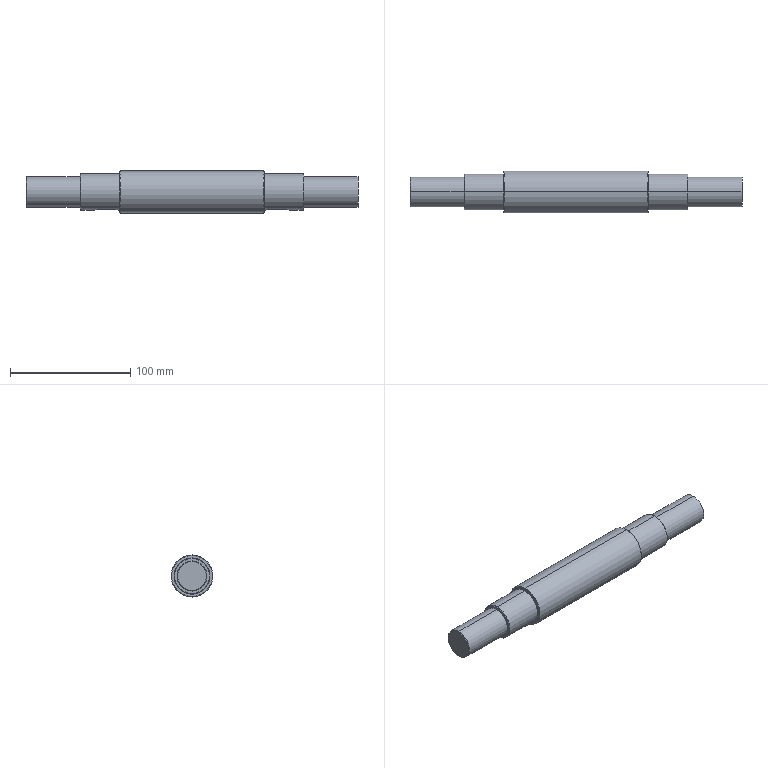Part | SolidWorks | features Chamfer 1, ICE 1, Revolution 1 | 1 solid | 38 faces | box 276 x 35 x 35 mm | volume 205103 mm3 | cylinder 16 | plane 12 | cone 10 | commonest cylinder face diameters 8 x6 25 x4 30 x4 35 x2
STEP:
#1=CARTESIAN_POINT('',(-65.,4.,-14.457));
#2=VERTEX_POINT('',#1);
#3=CARTESIAN_POINT('',(-61.,0.,-15.));
#4=VERTEX_POINT('',#3);
#5=CARTESIAN_POINT('',(-65.,4.,-14.457));
#6=CARTESIAN_POINT('',(-64.736,4.,-14.457));
#7=CARTESIAN_POINT('',(-64.476,3.974,-14.464));
#8=CARTESIAN_POINT('',(-63.962,3.872,-14.492));
#9=CARTESIAN_POINT('',(-63.707,3.794,-14.513));
#10=CARTESIAN_POINT('',(-63.224,3.594,-14.563));
#11=CARTESIAN_POINT('',(-62.995,3.471,-14.594));
#12=CARTESIAN_POINT('',(-62.558,3.179,-14.66));
#13=CARTESIAN_POINT('',(-62.356,3.013,-14.695));
#14=CARTESIAN_POINT('',(-61.989,2.646,-14.766));
#15=CARTESIAN_POINT('',(-61.822,2.443,-14.801));
#16=CARTESIAN_POINT('',(-61.531,2.008,-14.867));
#17=CARTESIAN_POINT('',(-61.408,1.779,-14.896));
#18=CARTESIAN_POINT('',(-61.207,1.297,-14.946));
#19=CARTESIAN_POINT('',(-61.129,1.042,-14.966));
#20=CARTESIAN_POINT('',(-61.026,0.527,-14.993));
#21=CARTESIAN_POINT('',(-61.,0.2655,-15.));
#22=CARTESIAN_POINT('',(-61.,0.,-15.));
#23=B_SPLINE_CURVE_WITH_KNOTS('',3,(#5,#6,#7,#8,#9,#10,#11,#12,#13,#14,#15,#16,#17,#18,#19,#20,#21,#22),.UNSPECIFIED.,.F.,.F.,(4,2,2,2,2,2,2,2,4),(0.01884,0.01963,0.02041,0.0212,0.02198,0.02277,0.02355,0.02434,0.02512),.UNSPECIFIED.);
#24=EDGE_CURVE('',#2,#4,#23,.T.);
#25=ORIENTED_EDGE('',*,*,#24,.T.);
#26=CARTESIAN_POINT('',(-61.,0.,-11.));
#27=VERTEX_POINT('',#26);
#28=CARTESIAN_POINT('',(-61.,0.,-21.));
#29=DIRECTION('',(0.,0.,1.));
#30=VECTOR('',#29,1000.);
#31=LINE('',#28,#30);
#32=EDGE_CURVE('',#4,#27,#31,.T.);
#33=ORIENTED_EDGE('',*,*,#32,.T.);
#34=CARTESIAN_POINT('',(-65.,4.,-11.));
#35=VERTEX_POINT('',#34);
#36=CARTESIAN_POINT('',(-65.,0.,-11.));
#37=DIRECTION('',(0.,0.,1.));
#38=DIRECTION('',(1.,0.,0.));
#39=AXIS2_PLACEMENT_3D('',#36,#37,#38);
#40=CIRCLE('',#39,4.);
#41=EDGE_CURVE('',#27,#35,#40,.T.);
#42=ORIENTED_EDGE('',*,*,#41,.T.);
#43=CARTESIAN_POINT('',(-65.,4.,-21.));
#44=DIRECTION('',(0.,0.,1.));
#45=VECTOR('',#44,1000.);
#46=LINE('',#43,#45);
#47=EDGE_CURVE('',#2,#35,#46,.T.);
#48=ORIENTED_EDGE('',*,*,#47,.F.);
#49=EDGE_LOOP('',(#25,#33,#42,#48));
#50=FACE_OUTER_BOUND('',#49,.T.);
#51=CARTESIAN_POINT('',(-65.,0.,-21.));
#52=DIRECTION('',(0.,0.,1.));
#53=DIRECTION('',(1.,0.,0.));
#54=AXIS2_PLACEMENT_3D('',#51,#52,#53);
#55=CYLINDRICAL_SURFACE('',#54,4.);
#56=ADVANCED_FACE('',(#50),#55,.F.);
#57=CARTESIAN_POINT('',(77.,4.,-14.457));
#58=VERTEX_POINT('',#57);
#59=CARTESIAN_POINT('',(81.,0.,-15.));
#60=VERTEX_POINT('',#59);
#61=CARTESIAN_POINT('',(77.,4.,-14.457));
#62=CARTESIAN_POINT('',(77.264,4.,-14.457));
#63=CARTESIAN_POINT('',(77.524,3.974,-14.464));
#64=CARTESIAN_POINT('',(78.038,3.872,-14.492));
#65=CARTESIAN_POINT('',(78.293,3.794,-14.513));
#66=CARTESIAN_POINT('',(78.776,3.594,-14.563));
#67=CARTESIAN_POINT('',(79.005,3.471,-14.594));
#68=CARTESIAN_POINT('',(79.442,3.179,-14.66));
#69=CARTESIAN_POINT('',(79.644,3.013,-14.695));
#70=CARTESIAN_POINT('',(80.011,2.646,-14.766));
#71=CARTESIAN_POINT('',(80.178,2.443,-14.801));
#72=CARTESIAN_POINT('',(80.469,2.008,-14.867));
#73=CARTESIAN_POINT('',(80.592,1.779,-14.896));
#74=CARTESIAN_POINT('',(80.793,1.297,-14.946));
#75=CARTESIAN_POINT('',(80.871,1.042,-14.966));
#76=CARTESIAN_POINT('',(80.974,0.527,-14.993));
#77=CARTESIAN_POINT('',(81.,0.2655,-15.));
#78=CARTESIAN_POINT('',(81.,0.,-15.));
#79=B_SPLINE_CURVE_WITH_KNOTS('',3,(#61,#62,#63,#64,#65,#66,#67,#68,#69,#70,#71,#72,#73,#74,#75,#76,#77,#78),.UNSPECIFIED.,.F.,.F.,(4,2,2,2,2,2,2,2,4),(0.01884,0.01963,0.02041,0.0212,0.02198,0.02277,0.02355,0.02434,0.02512),.UNSPECIFIED.);
#80=EDGE_CURVE('',#58,#60,#79,.T.);
#81=ORIENTED_EDGE('',*,*,#80,.T.);
#82=CARTESIAN_POINT('',(81.,0.,-11.));
#83=VERTEX_POINT('',#82);
#84=CARTESIAN_POINT('',(81.,0.,-21.));
#85=DIRECTION('',(0.,0.,1.));
#86=VECTOR('',#85,1000.);
#87=LINE('',#84,#86);
#88=EDGE_CURVE('',#60,#83,#87,.T.);
#89=ORIENTED_EDGE('',*,*,#88,.T.);
#90=CARTESIAN_POINT('',(77.,4.,-11.));
#91=VERTEX_POINT('',#90);
#92=CARTESIAN_POINT('',(77.,0.,-11.));
#93=DIRECTION('',(0.,0.,1.));
#94=DIRECTION('',(1.,0.,0.));
#95=AXIS2_PLACEMENT_3D('',#92,#93,#94);
#96=CIRCLE('',#95,4.);
#97=EDGE_CURVE('',#83,#91,#96,.T.);
#98=ORIENTED_EDGE('',*,*,#97,.T.);
#99=CARTESIAN_POINT('',(77.,4.,-21.));
#100=DIRECTION('',(0.,0.,1.));
#101=VECTOR('',#100,1000.);
#102=LINE('',#99,#101);
#103=EDGE_CURVE('',#58,#91,#102,.T.);
#104=ORIENTED_EDGE('',*,*,#103,.F.);
#105=EDGE_LOOP('',(#81,#89,#98,#104));
#106=FACE_OUTER_BOUND('',#105,.T.);
#107=CARTESIAN_POINT('',(77.,0.,-21.));
#108=DIRECTION('',(0.,0.,1.));
#109=DIRECTION('',(1.,0.,0.));
#110=AXIS2_PLACEMENT_3D('',#107,#108,#109);
#111=CYLINDRICAL_SURFACE('',#110,4.);
#112=ADVANCED_FACE('',(#106),#111,.F.);
#113=CARTESIAN_POINT('',(60.,0.,-17.));
#114=VERTEX_POINT('',#113);
#115=CARTESIAN_POINT('',(60.,0.,17.));
#116=VERTEX_POINT('',#115);
#117=CARTESIAN_POINT('',(60.,0.,0.));
#118=DIRECTION('',(1.,0.,0.));
#119=DIRECTION('',(0.,0.,-1.));
#120=AXIS2_PLACEMENT_3D('',#117,#118,#119);
#121=CIRCLE('',#120,17.);
#122=EDGE_CURVE('',#114,#116,#121,.T.);
#123=ORIENTED_EDGE('',*,*,#122,.F.);
#124=CARTESIAN_POINT('',(59.5,0.,-17.5));
#125=VERTEX_POINT('',#124);
#126=CARTESIAN_POINT('',(59.5,0.,-17.5));
#127=DIRECTION('',(-0.7071,0.,-0.7071));
#128=VECTOR('',#127,1000.);
#129=LINE('',#126,#128);
#130=EDGE_CURVE('',#114,#125,#129,.T.);
#131=ORIENTED_EDGE('',*,*,#130,.T.);
#132=CARTESIAN_POINT('',(59.5,0.,17.5));
#133=VERTEX_POINT('',#132);
#134=CARTESIAN_POINT('',(59.5,0.,0.));
#135=DIRECTION('',(-1.,0.,0.));
#136=DIRECTION('',(0.,0.,-1.));
#137=AXIS2_PLACEMENT_3D('',#134,#135,#136);
#138=CIRCLE('',#137,17.5);
#139=EDGE_CURVE('',#133,#125,#138,.T.);
#140=ORIENTED_EDGE('',*,*,#139,.F.);
#141=CARTESIAN_POINT('',(59.5,0.,17.5));
#142=DIRECTION('',(-0.7071,0.,0.7071));
#143=VECTOR('',#142,1000.);
#144=LINE('',#141,#143);
#145=EDGE_CURVE('',#116,#133,#144,.T.);
#146=ORIENTED_EDGE('',*,*,#145,.F.);
#147=EDGE_LOOP('',(#123,#131,#140,#146));
#148=FACE_OUTER_BOUND('',#147,.T.);
#149=CARTESIAN_POINT('',(59.5,0.,0.));
#150=DIRECTION('',(-1.,0.,0.));
#151=DIRECTION('',(0.,0.,1.));
#152=AXIS2_PLACEMENT_3D('',#149,#150,#151);
#153=CONICAL_SURFACE('',#152,17.5,0.7854);
#154=ADVANCED_FACE('',(#148),#153,.T.);
#155=CARTESIAN_POINT('',(93.,0.,-14.5));
#156=VERTEX_POINT('',#155);
#157=CARTESIAN_POINT('',(93.,0.,14.5));
#158=VERTEX_POINT('',#157);
#159=CARTESIAN_POINT('',(93.,0.,0.));
#160=DIRECTION('',(1.,0.,0.));
#161=DIRECTION('',(0.,0.,-1.));
#162=AXIS2_PLACEMENT_3D('',#159,#160,#161);
#163=CIRCLE('',#162,14.5);
#164=EDGE_CURVE('',#156,#158,#163,.T.);
#165=ORIENTED_EDGE('',*,*,#164,.F.);
#166=CARTESIAN_POINT('',(92.5,0.,-15.));
#167=VERTEX_POINT('',#166);
#168=CARTESIAN_POINT('',(92.5,0.,-15.));
#169=DIRECTION('',(-0.7071,0.,-0.7071));
#170=VECTOR('',#169,1000.);
#171=LINE('',#168,#170);
#172=EDGE_CURVE('',#156,#167,#171,.T.);
#173=ORIENTED_EDGE('',*,*,#172,.T.);
#174=CARTESIAN_POINT('',(92.5,0.,15.));
#175=VERTEX_POINT('',#174);
#176=CARTESIAN_POINT('',(92.5,0.,0.));
#177=DIRECTION('',(-1.,0.,0.));
#178=DIRECTION('',(0.,0.,-1.));
#179=AXIS2_PLACEMENT_3D('',#176,#177,#178);
#180=CIRCLE('',#179,15.);
#181=EDGE_CURVE('',#175,#167,#180,.T.);
#182=ORIENTED_EDGE('',*,*,#181,.F.);
#183=CARTESIAN_POINT('',(92.5,0.,15.));
#184=DIRECTION('',(-0.7071,0.,0.7071));
#185=VECTOR('',#184,1000.);
#186=LINE('',#183,#185);
#187=EDGE_CURVE('',#158,#175,#186,.T.);
#188=ORIENTED_EDGE('',*,*,#187,.F.);
#189=EDGE_LOOP('',(#165,#173,#182,#188));
#190=FACE_OUTER_BOUND('',#189,.T.);
#191=CARTESIAN_POINT('',(92.5,0.,0.));
#192=DIRECTION('',(-1.,0.,0.));
#193=DIRECTION('',(0.,0.,1.));
#194=AXIS2_PLACEMENT_3D('',#191,#192,#193);
#195=CONICAL_SURFACE('',#194,15.,0.7854);
#196=ADVANCED_FACE('',(#190),#195,.T.);
#197=CARTESIAN_POINT('',(-60.,0.,17.));
#198=VERTEX_POINT('',#197);
#199=CARTESIAN_POINT('',(-60.,0.,-17.));
#200=VERTEX_POINT('',#199);
#201=CARTESIAN_POINT('',(-60.,0.,0.));
#202=DIRECTION('',(-1.,0.,0.));
#203=DIRECTION('',(0.,0.,1.));
#204=AXIS2_PLACEMENT_3D('',#201,#202,#203);
#205=CIRCLE('',#204,17.);
#206=EDGE_CURVE('',#198,#200,#205,.T.);
#207=ORIENTED_EDGE('',*,*,#206,.F.);
#208=CARTESIAN_POINT('',(-59.5,0.,17.5));
#209=VERTEX_POINT('',#208);
#210=CARTESIAN_POINT('',(-60.,0.,17.));
#211=DIRECTION('',(0.7071,0.,0.7071));
#212=VECTOR('',#211,1000.);
#213=LINE('',#210,#212);
#214=EDGE_CURVE('',#198,#209,#213,.T.);
#215=ORIENTED_EDGE('',*,*,#214,.T.);
#216=CARTESIAN_POINT('',(-59.5,0.,-17.5));
#217=VERTEX_POINT('',#216);
#218=CARTESIAN_POINT('',(-59.5,0.,0.));
#219=DIRECTION('',(1.,0.,0.));
#220=DIRECTION('',(0.,0.,1.));
#221=AXIS2_PLACEMENT_3D('',#218,#219,#220);
#222=CIRCLE('',#221,17.5);
#223=EDGE_CURVE('',#217,#209,#222,.T.);
#224=ORIENTED_EDGE('',*,*,#223,.F.);
#225=CARTESIAN_POINT('',(-60.,0.,-17.));
#226=DIRECTION('',(0.7071,0.,-0.7071));
#227=VECTOR('',#226,1000.);
#228=LINE('',#225,#227);
#229=EDGE_CURVE('',#200,#217,#228,.T.);
#230=ORIENTED_EDGE('',*,*,#229,.F.);
#231=EDGE_LOOP('',(#207,#215,#224,#230));
#232=FACE_OUTER_BOUND('',#231,.T.);
#233=CARTESIAN_POINT('',(-60.,0.,0.));
#234=DIRECTION('',(1.,0.,0.));
#235=DIRECTION('',(0.,0.,-1.));
#236=AXIS2_PLACEMENT_3D('',#233,#234,#235);
#237=CONICAL_SURFACE('',#236,17.,0.7854);
#238=ADVANCED_FACE('',(#232),#237,.T.);
#239=CARTESIAN_POINT('',(-93.,0.,14.5));
#240=VERTEX_POINT('',#239);
#241=CARTESIAN_POINT('',(-93.,0.,-14.5));
#242=VERTEX_POINT('',#241);
#243=CARTESIAN_POINT('',(-93.,0.,0.));
#244=DIRECTION('',(-1.,0.,0.));
#245=DIRECTION('',(0.,0.,1.));
#246=AXIS2_PLACEMENT_3D('',#243,#244,#245);
#247=CIRCLE('',#246,14.5);
#248=EDGE_CURVE('',#240,#242,#247,.T.);
#249=ORIENTED_EDGE('',*,*,#248,.F.);
#250=CARTESIAN_POINT('',(-92.5,0.,15.));
#251=VERTEX_POINT('',#250);
#252=CARTESIAN_POINT('',(-93.,0.,14.5));
#253=DIRECTION('',(0.7071,0.,0.7071));
#254=VECTOR('',#253,1000.);
#255=LINE('',#252,#254);
#256=EDGE_CURVE('',#240,#251,#255,.T.);
#257=ORIENTED_EDGE('',*,*,#256,.T.);
#258=CARTESIAN_POINT('',(-92.5,0.,-15.));
#259=VERTEX_POINT('',#258);
#260=CARTESIAN_POINT('',(-92.5,0.,0.));
#261=DIRECTION('',(1.,0.,0.));
#262=DIRECTION('',(0.,0.,1.));
#263=AXIS2_PLACEMENT_3D('',#260,#261,#262);
#264=CIRCLE('',#263,15.);
#265=EDGE_CURVE('',#259,#251,#264,.T.);
#266=ORIENTED_EDGE('',*,*,#265,.F.);
#267=CARTESIAN_POINT('',(-93.,0.,-14.5));
#268=DIRECTION('',(0.7071,0.,-0.7071));
#269=VECTOR('',#268,1000.);
#270=LINE('',#267,#269);
#271=EDGE_CURVE('',#242,#259,#270,.T.);
#272=ORIENTED_EDGE('',*,*,#271,.F.);
#273=EDGE_LOOP('',(#249,#257,#266,#272));
#274=FACE_OUTER_BOUND('',#273,.T.);
#275=CARTESIAN_POINT('',(-93.,0.,0.));
#276=DIRECTION('',(1.,0.,0.));
#277=DIRECTION('',(0.,0.,-1.));
#278=AXIS2_PLACEMENT_3D('',#275,#276,#277);
#279=CONICAL_SURFACE('',#278,14.5,0.7854);
#280=ADVANCED_FACE('',(#274),#279,.T.);
#281=CARTESIAN_POINT('',(-138.,0.,12.));
#282=VERTEX_POINT('',#281);
#283=CARTESIAN_POINT('',(-138.,0.,-12.));
#284=VERTEX_POINT('',#283);
#285=CARTESIAN_POINT('',(-138.,0.,0.));
#286=DIRECTION('',(-1.,0.,0.));
#287=DIRECTION('',(0.,0.,1.));
#288=AXIS2_PLACEMENT_3D('',#285,#286,#287);
#289=CIRCLE('',#288,12.);
#290=EDGE_CURVE('',#282,#284,#289,.T.);
#291=ORIENTED_EDGE('',*,*,#290,.F.);
#292=CARTESIAN_POINT('',(-137.5,0.,12.5));
#293=VERTEX_POINT('',#292);
#294=CARTESIAN_POINT('',(-138.,0.,12.));
#295=DIRECTION('',(0.7071,0.,0.7071));
#296=VECTOR('',#295,1000.);
#297=LINE('',#294,#296);
#298=EDGE_CURVE('',#282,#293,#297,.T.);
#299=ORIENTED_EDGE('',*,*,#298,.T.);
#300=CARTESIAN_POINT('',(-137.5,0.,-12.5));
#301=VERTEX_POINT('',#300);
#302=CARTESIAN_POINT('',(-137.5,0.,0.));
#303=DIRECTION('',(1.,0.,0.));
#304=DIRECTION('',(0.,0.,1.));
#305=AXIS2_PLACEMENT_3D('',#302,#303,#304);
#306=CIRCLE('',#305,12.5);
#307=EDGE_CURVE('',#301,#293,#306,.T.);
#308=ORIENTED_EDGE('',*,*,#307,.F.);
#309=CARTESIAN_POINT('',(-138.,0.,-12.));
#310=DIRECTION('',(0.7071,0.,-0.7071));
#311=VECTOR('',#310,1000.);
#312=LINE('',#309,#311);
#313=EDGE_CURVE('',#284,#301,#312,.T.);
#314=ORIENTED_EDGE('',*,*,#313,.F.);
#315=EDGE_LOOP('',(#291,#299,#308,#314));
#316=FACE_OUTER_BOUND('',#315,.T.);
#317=CARTESIAN_POINT('',(-138.,0.,0.));
#318=DIRECTION('',(1.,0.,0.));
#319=DIRECTION('',(0.,0.,-1.));
#320=AXIS2_PLACEMENT_3D('',#317,#318,#319);
#321=CONICAL_SURFACE('',#320,12.,0.7854);
#322=ADVANCED_FACE('',(#316),#321,.T.);
#323=ORIENTED_EDGE('',*,*,#181,.T.);
#324=CARTESIAN_POINT('',(70.,0.,-15.));
#325=DIRECTION('',(-1.,0.,0.));
#326=VECTOR('',#325,1000.);
#327=LINE('',#324,#326);
#328=EDGE_CURVE('',#167,#60,#327,.T.);
#329=ORIENTED_EDGE('',*,*,#328,.T.);
#330=ORIENTED_EDGE('',*,*,#80,.F.);
#331=CARTESIAN_POINT('',(65.,4.,-14.457));
#332=VERTEX_POINT('',#331);
#333=CARTESIAN_POINT('',(70.,4.,-14.457));
#334=DIRECTION('',(1.,0.,0.));
#335=VECTOR('',#334,1000.);
#336=LINE('',#333,#335);
#337=EDGE_CURVE('',#332,#58,#336,.T.);
#338=ORIENTED_EDGE('',*,*,#337,.F.);
#339=CARTESIAN_POINT('',(61.,0.,-15.));
#340=VERTEX_POINT('',#339);
#341=CARTESIAN_POINT('',(61.,0.,-15.));
#342=CARTESIAN_POINT('',(61.,0.262,-15.));
#343=CARTESIAN_POINT('',(61.026,0.5282,-14.993));
#344=CARTESIAN_POINT('',(61.129,1.042,-14.966));
#345=CARTESIAN_POINT('',(61.205,1.292,-14.946));
#346=CARTESIAN_POINT('',(61.508,2.02,-14.871));
#347=CARTESIAN_POINT('',(61.802,2.459,-14.802));
#348=CARTESIAN_POINT('',(62.357,3.014,-14.695));
#349=CARTESIAN_POINT('',(62.557,3.178,-14.66));
#350=CARTESIAN_POINT('',(62.989,3.467,-14.594));
#351=CARTESIAN_POINT('',(63.223,3.593,-14.564));
#352=CARTESIAN_POINT('',(63.705,3.794,-14.513));
#353=CARTESIAN_POINT('',(63.954,3.87,-14.492));
#354=CARTESIAN_POINT('',(64.469,3.973,-14.464));
#355=CARTESIAN_POINT('',(64.735,4.,-14.457));
#356=CARTESIAN_POINT('',(65.,4.,-14.457));
#357=B_SPLINE_CURVE_WITH_KNOTS('',3,(#341,#342,#343,#344,#345,#346,#347,#348,#349,#350,#351,#352,#353,#354,#355,#356),.UNSPECIFIED.,.F.,.F.,(4,2,2,2,2,2,2,4),(0.006283,0.007068,0.007852,0.009421,0.01021,0.01099,0.01177,0.01256),.UNSPECIFIED.);
#358=EDGE_CURVE('',#340,#332,#357,.T.);
#359=ORIENTED_EDGE('',*,*,#358,.F.);
#360=CARTESIAN_POINT('',(60.,0.,-15.));
#361=VERTEX_POINT('',#360);
#362=CARTESIAN_POINT('',(70.,0.,-15.));
#363=DIRECTION('',(-1.,0.,0.));
#364=VECTOR('',#363,1000.);
#365=LINE('',#362,#364);
#366=EDGE_CURVE('',#340,#361,#365,.T.);
#367=ORIENTED_EDGE('',*,*,#366,.T.);
#368=CARTESIAN_POINT('',(60.,0.,15.));
#369=VERTEX_POINT('',#368);
#370=CARTESIAN_POINT('',(60.,0.,0.));
#371=DIRECTION('',(-1.,0.,0.));
#372=DIRECTION('',(0.,0.,1.));
#373=AXIS2_PLACEMENT_3D('',#370,#371,#372);
#374=CIRCLE('',#373,15.);
#375=EDGE_CURVE('',#369,#361,#374,.T.);
#376=ORIENTED_EDGE('',*,*,#375,.F.);
#377=CARTESIAN_POINT('',(70.,0.,15.));
#378=DIRECTION('',(-1.,0.,0.));
#379=VECTOR('',#378,1000.);
#380=LINE('',#377,#379);
#381=EDGE_CURVE('',#175,#369,#380,.T.);
#382=ORIENTED_EDGE('',*,*,#381,.F.);
#383=EDGE_LOOP('',(#323,#329,#330,#338,#359,#367,#376,#382));
#384=FACE_OUTER_BOUND('',#383,.T.);
#385=CARTESIAN_POINT('',(70.,0.,0.));
#386=DIRECTION('',(-1.,0.,0.));
#387=DIRECTION('',(0.,0.,1.));
#388=AXIS2_PLACEMENT_3D('',#385,#386,#387);
#389=CYLINDRICAL_SURFACE('',#388,15.);
#390=ADVANCED_FACE('',(#384),#389,.T.);
#391=CARTESIAN_POINT('',(138.,0.,12.5));
#392=VERTEX_POINT('',#391);
#393=CARTESIAN_POINT('',(138.,0.,-12.5));
#394=VERTEX_POINT('',#393);
#395=CARTESIAN_POINT('',(138.,0.,0.));
#396=DIRECTION('',(-1.,0.,0.));
#397=DIRECTION('',(0.,0.,1.));
#398=AXIS2_PLACEMENT_3D('',#395,#396,#397);
#399=CIRCLE('',#398,12.5);
#400=EDGE_CURVE('',#392,#394,#399,.T.);
#401=ORIENTED_EDGE('',*,*,#400,.T.);
#402=CARTESIAN_POINT('',(93.,0.,-12.5));
#403=VERTEX_POINT('',#402);
#404=CARTESIAN_POINT('',(70.,0.,-12.5));
#405=DIRECTION('',(-1.,0.,0.));
#406=VECTOR('',#405,1000.);
#407=LINE('',#404,#406);
#408=EDGE_CURVE('',#394,#403,#407,.T.);
#409=ORIENTED_EDGE('',*,*,#408,.T.);
#410=CARTESIAN_POINT('',(93.,0.,12.5));
#411=VERTEX_POINT('',#410);
#412=CARTESIAN_POINT('',(93.,0.,0.));
#413=DIRECTION('',(-1.,0.,0.));
#414=DIRECTION('',(0.,0.,1.));
#415=AXIS2_PLACEMENT_3D('',#412,#413,#414);
#416=CIRCLE('',#415,12.5);
#417=EDGE_CURVE('',#411,#403,#416,.T.);
#418=ORIENTED_EDGE('',*,*,#417,.F.);
#419=CARTESIAN_POINT('',(70.,0.,12.5));
#420=DIRECTION('',(-1.,0.,0.));
#421=VECTOR('',#420,1000.);
#422=LINE('',#419,#421);
#423=EDGE_CURVE('',#392,#411,#422,.T.);
#424=ORIENTED_EDGE('',*,*,#423,.F.);
#425=EDGE_LOOP('',(#401,#409,#418,#424));
#426=FACE_OUTER_BOUND('',#425,.T.);
#427=CARTESIAN_POINT('',(70.,0.,0.));
#428=DIRECTION('',(-1.,0.,0.));
#429=DIRECTION('',(0.,0.,1.));
#430=AXIS2_PLACEMENT_3D('',#427,#428,#429);
#431=CYLINDRICAL_SURFACE('',#430,12.5);
#432=ADVANCED_FACE('',(#426),#431,.T.);
#433=CARTESIAN_POINT('',(-93.,0.,12.5));
#434=VERTEX_POINT('',#433);
#435=CARTESIAN_POINT('',(-93.,0.,-12.5));
#436=VERTEX_POINT('',#435);
#437=CARTESIAN_POINT('',(-93.,0.,0.));
#438=DIRECTION('',(-1.,0.,0.));
#439=DIRECTION('',(0.,0.,1.));
#440=AXIS2_PLACEMENT_3D('',#437,#438,#439);
#441=CIRCLE('',#440,12.5);
#442=EDGE_CURVE('',#434,#436,#441,.T.);
#443=ORIENTED_EDGE('',*,*,#442,.T.);
#444=CARTESIAN_POINT('',(70.,0.,-12.5));
#445=DIRECTION('',(-1.,0.,0.));
#446=VECTOR('',#445,1000.);
#447=LINE('',#444,#446);
#448=EDGE_CURVE('',#436,#301,#447,.T.);
#449=ORIENTED_EDGE('',*,*,#448,.T.);
#450=ORIENTED_EDGE('',*,*,#307,.T.);
#451=CARTESIAN_POINT('',(70.,0.,12.5));
#452=DIRECTION('',(-1.,0.,0.));
#453=VECTOR('',#452,1000.);
#454=LINE('',#451,#453);
#455=EDGE_CURVE('',#434,#293,#454,.T.);
#456=ORIENTED_EDGE('',*,*,#455,.F.);
#457=EDGE_LOOP('',(#443,#449,#450,#456));
#458=FACE_OUTER_BOUND('',#457,.T.);
#459=CARTESIAN_POINT('',(70.,0.,0.));
#460=DIRECTION('',(-1.,0.,0.));
#461=DIRECTION('',(0.,0.,1.));
#462=AXIS2_PLACEMENT_3D('',#459,#460,#461);
#463=CYLINDRICAL_SURFACE('',#462,12.5);
#464=ADVANCED_FACE('',(#458),#463,.T.);
#465=CARTESIAN_POINT('',(-60.,0.,15.));
#466=VERTEX_POINT('',#465);
#467=CARTESIAN_POINT('',(-60.,0.,-15.));
#468=VERTEX_POINT('',#467);
#469=CARTESIAN_POINT('',(-60.,0.,0.));
#470=DIRECTION('',(-1.,0.,0.));
#471=DIRECTION('',(0.,0.,1.));
#472=AXIS2_PLACEMENT_3D('',#469,#470,#471);
#473=CIRCLE('',#472,15.);
#474=EDGE_CURVE('',#466,#468,#473,.T.);
#475=ORIENTED_EDGE('',*,*,#474,.T.);
#476=CARTESIAN_POINT('',(70.,0.,-15.));
#477=DIRECTION('',(-1.,0.,0.));
#478=VECTOR('',#477,1000.);
#479=LINE('',#476,#478);
#480=EDGE_CURVE('',#468,#4,#479,.T.);
#481=ORIENTED_EDGE('',*,*,#480,.T.);
#482=ORIENTED_EDGE('',*,*,#24,.F.);
#483=CARTESIAN_POINT('',(-77.,4.,-14.457));
#484=VERTEX_POINT('',#483);
#485=CARTESIAN_POINT('',(70.,4.,-14.457));
#486=DIRECTION('',(1.,0.,0.));
#487=VECTOR('',#486,1000.);
#488=LINE('',#485,#487);
#489=EDGE_CURVE('',#484,#2,#488,.T.);
#490=ORIENTED_EDGE('',*,*,#489,.F.);
#491=CARTESIAN_POINT('',(-81.,0.,-15.));
#492=VERTEX_POINT('',#491);
#493=CARTESIAN_POINT('',(-81.,0.,-15.));
#494=CARTESIAN_POINT('',(-81.,0.262,-15.));
#495=CARTESIAN_POINT('',(-80.974,0.5282,-14.993));
#496=CARTESIAN_POINT('',(-80.871,1.042,-14.966));
#497=CARTESIAN_POINT('',(-80.795,1.292,-14.946));
#498=CARTESIAN_POINT('',(-80.492,2.02,-14.871));
#499=CARTESIAN_POINT('',(-80.198,2.459,-14.802));
#500=CARTESIAN_POINT('',(-79.643,3.014,-14.695));
#501=CARTESIAN_POINT('',(-79.443,3.178,-14.66));
#502=CARTESIAN_POINT('',(-79.011,3.467,-14.594));
#503=CARTESIAN_POINT('',(-78.777,3.593,-14.564));
#504=CARTESIAN_POINT('',(-78.295,3.794,-14.513));
#505=CARTESIAN_POINT('',(-78.046,3.87,-14.492));
#506=CARTESIAN_POINT('',(-77.531,3.973,-14.464));
#507=CARTESIAN_POINT('',(-77.265,4.,-14.457));
#508=CARTESIAN_POINT('',(-77.,4.,-14.457));
#509=B_SPLINE_CURVE_WITH_KNOTS('',3,(#493,#494,#495,#496,#497,#498,#499,#500,#501,#502,#503,#504,#505,#506,#507,#508),.UNSPECIFIED.,.F.,.F.,(4,2,2,2,2,2,2,4),(0.006283,0.007068,0.007852,0.009421,0.01021,0.01099,0.01177,0.01256),.UNSPECIFIED.);
#510=EDGE_CURVE('',#492,#484,#509,.T.);
#511=ORIENTED_EDGE('',*,*,#510,.F.);
#512=CARTESIAN_POINT('',(70.,0.,-15.));
#513=DIRECTION('',(-1.,0.,0.));
#514=VECTOR('',#513,1000.);
#515=LINE('',#512,#514);
#516=EDGE_CURVE('',#492,#259,#515,.T.);
#517=ORIENTED_EDGE('',*,*,#516,.T.);
#518=ORIENTED_EDGE('',*,*,#265,.T.);
#519=CARTESIAN_POINT('',(70.,0.,15.));
#520=DIRECTION('',(-1.,0.,0.));
#521=VECTOR('',#520,1000.);
#522=LINE('',#519,#521);
#523=EDGE_CURVE('',#466,#251,#522,.T.);
#524=ORIENTED_EDGE('',*,*,#523,.F.);
#525=EDGE_LOOP('',(#475,#481,#482,#490,#511,#517,#518,#524));
#526=FACE_OUTER_BOUND('',#525,.T.);
#527=CARTESIAN_POINT('',(70.,0.,0.));
#528=DIRECTION('',(-1.,0.,0.));
#529=DIRECTION('',(0.,0.,1.));
#530=AXIS2_PLACEMENT_3D('',#527,#528,#529);
#531=CYLINDRICAL_SURFACE('',#530,15.);
#532=ADVANCED_FACE('',(#526),#531,.T.);
#533=ORIENTED_EDGE('',*,*,#139,.T.);
#534=CARTESIAN_POINT('',(70.,0.,-17.5));
#535=DIRECTION('',(-1.,0.,0.));
#536=VECTOR('',#535,1000.);
#537=LINE('',#534,#536);
#538=EDGE_CURVE('',#125,#217,#537,.T.);
#539=ORIENTED_EDGE('',*,*,#538,.T.);
#540=ORIENTED_EDGE('',*,*,#223,.T.);
#541=CARTESIAN_POINT('',(70.,0.,17.5));
#542=DIRECTION('',(-1.,0.,0.));
#543=VECTOR('',#542,1000.);
#544=LINE('',#541,#543);
#545=EDGE_CURVE('',#133,#209,#544,.T.);
#546=ORIENTED_EDGE('',*,*,#545,.F.);
#547=EDGE_LOOP('',(#533,#539,#540,#546));
#548=FACE_OUTER_BOUND('',#547,.T.);
#549=CARTESIAN_POINT('',(70.,0.,0.));
#550=DIRECTION('',(-1.,0.,0.));
#551=DIRECTION('',(0.,0.,1.));
#552=AXIS2_PLACEMENT_3D('',#549,#550,#551);
#553=CYLINDRICAL_SURFACE('',#552,17.5);
#554=ADVANCED_FACE('',(#548),#553,.T.);
#555=CARTESIAN_POINT('',(60.,0.,0.));
#556=DIRECTION('',(1.,0.,0.));
#557=DIRECTION('',(0.,0.,-1.));
#558=AXIS2_PLACEMENT_3D('',#555,#556,#557);
#559=CIRCLE('',#558,17.);
#560=EDGE_CURVE('',#116,#114,#559,.T.);
#561=ORIENTED_EDGE('',*,*,#560,.T.);
#562=ORIENTED_EDGE('',*,*,#122,.T.);
#563=EDGE_LOOP('',(#561,#562));
#564=FACE_OUTER_BOUND('',#563,.T.);
#565=ORIENTED_EDGE('',*,*,#375,.T.);
#566=CARTESIAN_POINT('',(60.,0.,0.));
#567=DIRECTION('',(-1.,0.,0.));
#568=DIRECTION('',(0.,0.,1.));
#569=AXIS2_PLACEMENT_3D('',#566,#567,#568);
#570=CIRCLE('',#569,15.);
#571=EDGE_CURVE('',#361,#369,#570,.T.);
#572=ORIENTED_EDGE('',*,*,#571,.T.);
#573=EDGE_LOOP('',(#565,#572));
#574=FACE_BOUND('',#573,.T.);
#575=CARTESIAN_POINT('',(60.,17.5,0.));
#576=DIRECTION('',(1.,0.,0.));
#577=DIRECTION('',(0.,0.,-1.));
#578=AXIS2_PLACEMENT_3D('',#575,#576,#577);
#579=PLANE('',#578);
#580=ADVANCED_FACE('',(#564,#574),#579,.T.);
#581=ORIENTED_EDGE('',*,*,#538,.F.);
#582=CARTESIAN_POINT('',(59.5,0.,0.));
#583=DIRECTION('',(-1.,0.,0.));
#584=DIRECTION('',(0.,0.,-1.));
#585=AXIS2_PLACEMENT_3D('',#582,#583,#584);
#586=CIRCLE('',#585,17.5);
#587=EDGE_CURVE('',#125,#133,#586,.T.);
#588=ORIENTED_EDGE('',*,*,#587,.T.);
#589=ORIENTED_EDGE('',*,*,#545,.T.);
#590=CARTESIAN_POINT('',(-59.5,0.,0.));
#591=DIRECTION('',(1.,0.,0.));
#592=DIRECTION('',(0.,0.,1.));
#593=AXIS2_PLACEMENT_3D('',#590,#591,#592);
#594=CIRCLE('',#593,17.5);
#595=EDGE_CURVE('',#209,#217,#594,.T.);
#596=ORIENTED_EDGE('',*,*,#595,.T.);
#597=EDGE_LOOP('',(#581,#588,#589,#596));
#598=FACE_OUTER_BOUND('',#597,.T.);
#599=CARTESIAN_POINT('',(70.,0.,0.));
#600=DIRECTION('',(-1.,0.,0.));
#601=DIRECTION('',(0.,0.,1.));
#602=AXIS2_PLACEMENT_3D('',#599,#600,#601);
#603=CYLINDRICAL_SURFACE('',#602,17.5);
#604=ADVANCED_FACE('',(#598),#603,.T.);
#605=CARTESIAN_POINT('',(-60.,0.,0.));
#606=DIRECTION('',(-1.,0.,0.));
#607=DIRECTION('',(0.,0.,1.));
#608=AXIS2_PLACEMENT_3D('',#605,#606,#607);
#609=CIRCLE('',#608,17.);
#610=EDGE_CURVE('',#200,#198,#609,.T.);
#611=ORIENTED_EDGE('',*,*,#610,.T.);
#612=ORIENTED_EDGE('',*,*,#206,.T.);
#613=EDGE_LOOP('',(#611,#612));
#614=FACE_OUTER_BOUND('',#613,.T.);
#615=ORIENTED_EDGE('',*,*,#474,.F.);
#616=CARTESIAN_POINT('',(-60.,0.,0.));
#617=DIRECTION('',(-1.,0.,0.));
#618=DIRECTION('',(0.,0.,1.));
#619=AXIS2_PLACEMENT_3D('',#616,#617,#618);
#620=CIRCLE('',#619,15.);
#621=EDGE_CURVE('',#468,#466,#620,.T.);
#622=ORIENTED_EDGE('',*,*,#621,.F.);
#623=EDGE_LOOP('',(#615,#622));
#624=FACE_BOUND('',#623,.T.);
#625=CARTESIAN_POINT('',(-60.,17.5,0.));
#626=DIRECTION('',(-1.,0.,0.));
#627=DIRECTION('',(0.,0.,1.));
#628=AXIS2_PLACEMENT_3D('',#625,#626,#627);
#629=PLANE('',#628);
#630=ADVANCED_FACE('',(#614,#624),#629,.T.);
#631=ORIENTED_EDGE('',*,*,#480,.F.);
#632=ORIENTED_EDGE('',*,*,#621,.T.);
#633=ORIENTED_EDGE('',*,*,#523,.T.);
#634=CARTESIAN_POINT('',(-92.5,0.,0.));
#635=DIRECTION('',(1.,0.,0.));
#636=DIRECTION('',(0.,0.,1.));
#637=AXIS2_PLACEMENT_3D('',#634,#635,#636);
#638=CIRCLE('',#637,15.);
#639=EDGE_CURVE('',#251,#259,#638,.T.);
#640=ORIENTED_EDGE('',*,*,#639,.T.);
#641=ORIENTED_EDGE('',*,*,#516,.F.);
#642=CARTESIAN_POINT('',(-77.,-4.,-14.457));
#643=VERTEX_POINT('',#642);
#644=CARTESIAN_POINT('',(-77.,-4.,-14.457));
#645=CARTESIAN_POINT('',(-77.266,-4.,-14.457));
#646=CARTESIAN_POINT('',(-77.527,-3.974,-14.464));
#647=CARTESIAN_POINT('',(-78.04,-3.871,-14.492));
#648=CARTESIAN_POINT('',(-78.294,-3.794,-14.513));
#649=CARTESIAN_POINT('',(-78.778,-3.593,-14.564));
#650=CARTESIAN_POINT('',(-79.008,-3.47,-14.594));
#651=CARTESIAN_POINT('',(-79.442,-3.179,-14.66));
#652=CARTESIAN_POINT('',(-79.646,-3.011,-14.696));
#653=CARTESIAN_POINT('',(-80.013,-2.644,-14.766));
#654=CARTESIAN_POINT('',(-80.178,-2.443,-14.801));
#655=CARTESIAN_POINT('',(-80.471,-2.006,-14.867));
#656=CARTESIAN_POINT('',(-80.594,-1.775,-14.897));
#657=CARTESIAN_POINT('',(-80.794,-1.293,-14.946));
#658=CARTESIAN_POINT('',(-80.871,-1.04,-14.966));
#659=CARTESIAN_POINT('',(-80.974,-0.5228,-14.993));
#660=CARTESIAN_POINT('',(-81.,-0.2623,-15.));
#661=CARTESIAN_POINT('',(-81.,0.,-15.));
#662=B_SPLINE_CURVE_WITH_KNOTS('',3,(#644,#645,#646,#647,#648,#649,#650,#651,#652,#653,#654,#655,#656,#657,#658,#659,#660,#661),.UNSPECIFIED.,.F.,.F.,(4,2,2,2,2,2,2,2,4),(0.,0.0007854,0.001571,0.002356,0.003142,0.003927,0.004712,0.005498,0.006283),.UNSPECIFIED.);
#663=EDGE_CURVE('',#643,#492,#662,.T.);
#664=ORIENTED_EDGE('',*,*,#663,.F.);
#665=CARTESIAN_POINT('',(-65.,-4.,-14.457));
#666=VERTEX_POINT('',#665);
#667=CARTESIAN_POINT('',(70.,-4.,-14.457));
#668=DIRECTION('',(-1.,0.,0.));
#669=VECTOR('',#668,1000.);
#670=LINE('',#667,#669);
#671=EDGE_CURVE('',#666,#643,#670,.T.);
#672=ORIENTED_EDGE('',*,*,#671,.F.);
#673=CARTESIAN_POINT('',(-61.,0.,-15.));
#674=CARTESIAN_POINT('',(-61.,-0.2657,-15.));
#675=CARTESIAN_POINT('',(-61.026,-0.5266,-14.993));
#676=CARTESIAN_POINT('',(-61.129,-1.04,-14.966));
#677=CARTESIAN_POINT('',(-61.206,-1.295,-14.946));
#678=CARTESIAN_POINT('',(-61.408,-1.779,-14.896));
#679=CARTESIAN_POINT('',(-61.531,-2.008,-14.867));
#680=CARTESIAN_POINT('',(-61.821,-2.442,-14.802));
#681=CARTESIAN_POINT('',(-61.989,-2.646,-14.766));
#682=CARTESIAN_POINT('',(-62.357,-3.013,-14.695));
#683=CARTESIAN_POINT('',(-62.558,-3.179,-14.66));
#684=CARTESIAN_POINT('',(-62.995,-3.471,-14.594));
#685=CARTESIAN_POINT('',(-63.226,-3.594,-14.563));
#686=CARTESIAN_POINT('',(-63.707,-3.794,-14.513));
#687=CARTESIAN_POINT('',(-63.96,-3.871,-14.492));
#688=CARTESIAN_POINT('',(-64.477,-3.974,-14.464));
#689=CARTESIAN_POINT('',(-64.738,-4.,-14.457));
#690=CARTESIAN_POINT('',(-65.,-4.,-14.457));
#691=B_SPLINE_CURVE_WITH_KNOTS('',3,(#673,#674,#675,#676,#677,#678,#679,#680,#681,#682,#683,#684,#685,#686,#687,#688,#689,#690),.UNSPECIFIED.,.F.,.F.,(4,2,2,2,2,2,2,2,4),(0.,0.0007854,0.001571,0.002356,0.003142,0.003927,0.004712,0.005498,0.006283),.UNSPECIFIED.);
#692=EDGE_CURVE('',#4,#666,#691,.T.);
#693=ORIENTED_EDGE('',*,*,#692,.F.);
#694=EDGE_LOOP('',(#631,#632,#633,#640,#641,#664,#672,#693));
#695=FACE_OUTER_BOUND('',#694,.T.);
#696=CARTESIAN_POINT('',(70.,0.,0.));
#697=DIRECTION('',(-1.,0.,0.));
#698=DIRECTION('',(0.,0.,1.));
#699=AXIS2_PLACEMENT_3D('',#696,#697,#698);
#700=CYLINDRICAL_SURFACE('',#699,15.);
#701=ADVANCED_FACE('',(#695),#700,.T.);
#702=CARTESIAN_POINT('',(-93.,0.,0.));
#703=DIRECTION('',(-1.,0.,0.));
#704=DIRECTION('',(0.,0.,1.));
#705=AXIS2_PLACEMENT_3D('',#702,#703,#704);
#706=CIRCLE('',#705,14.5);
#707=EDGE_CURVE('',#242,#240,#706,.T.);
#708=ORIENTED_EDGE('',*,*,#707,.T.);
#709=ORIENTED_EDGE('',*,*,#248,.T.);
#710=EDGE_LOOP('',(#708,#709));
#711=FACE_OUTER_BOUND('',#710,.T.);
#712=ORIENTED_EDGE('',*,*,#442,.F.);
#713=CARTESIAN_POINT('',(-93.,0.,0.));
#714=DIRECTION('',(-1.,0.,0.));
#715=DIRECTION('',(0.,0.,1.));
#716=AXIS2_PLACEMENT_3D('',#713,#714,#715);
#717=CIRCLE('',#716,12.5);
#718=EDGE_CURVE('',#436,#434,#717,.T.);
#719=ORIENTED_EDGE('',*,*,#718,.F.);
#720=EDGE_LOOP('',(#712,#719));
#721=FACE_BOUND('',#720,.T.);
#722=CARTESIAN_POINT('',(-93.,15.,0.));
#723=DIRECTION('',(-1.,0.,0.));
#724=DIRECTION('',(0.,0.,1.));
#725=AXIS2_PLACEMENT_3D('',#722,#723,#724);
#726=PLANE('',#725);
#727=ADVANCED_FACE('',(#711,#721),#726,.T.);
#728=ORIENTED_EDGE('',*,*,#448,.F.);
#729=ORIENTED_EDGE('',*,*,#718,.T.);
#730=ORIENTED_EDGE('',*,*,#455,.T.);
#731=CARTESIAN_POINT('',(-137.5,0.,0.));
#732=DIRECTION('',(1.,0.,0.));
#733=DIRECTION('',(0.,0.,1.));
#734=AXIS2_PLACEMENT_3D('',#731,#732,#733);
#735=CIRCLE('',#734,12.5);
#736=EDGE_CURVE('',#293,#301,#735,.T.);
#737=ORIENTED_EDGE('',*,*,#736,.T.);
#738=EDGE_LOOP('',(#728,#729,#730,#737));
#739=FACE_OUTER_BOUND('',#738,.T.);
#740=CARTESIAN_POINT('',(70.,0.,0.));
#741=DIRECTION('',(-1.,0.,0.));
#742=DIRECTION('',(0.,0.,1.));
#743=AXIS2_PLACEMENT_3D('',#740,#741,#742);
#744=CYLINDRICAL_SURFACE('',#743,12.5);
#745=ADVANCED_FACE('',(#739),#744,.T.);
#746=CARTESIAN_POINT('',(-138.,0.,0.));
#747=DIRECTION('',(-1.,0.,0.));
#748=DIRECTION('',(0.,0.,1.));
#749=AXIS2_PLACEMENT_3D('',#746,#747,#748);
#750=CIRCLE('',#749,12.);
#751=EDGE_CURVE('',#284,#282,#750,.T.);
#752=ORIENTED_EDGE('',*,*,#751,.T.);
#753=ORIENTED_EDGE('',*,*,#290,.T.);
#754=EDGE_LOOP('',(#752,#753));
#755=FACE_OUTER_BOUND('',#754,.T.);
#756=CARTESIAN_POINT('',(-138.,12.5,0.));
#757=DIRECTION('',(-1.,0.,0.));
#758=DIRECTION('',(0.,0.,1.));
#759=AXIS2_PLACEMENT_3D('',#756,#757,#758);
#760=PLANE('',#759);
#761=ADVANCED_FACE('',(#755),#760,.T.);
#762=ORIENTED_EDGE('',*,*,#400,.F.);
#763=CARTESIAN_POINT('',(138.,0.,0.));
#764=DIRECTION('',(-1.,0.,0.));
#765=DIRECTION('',(0.,0.,1.));
#766=AXIS2_PLACEMENT_3D('',#763,#764,#765);
#767=CIRCLE('',#766,12.5);
#768=EDGE_CURVE('',#394,#392,#767,.T.);
#769=ORIENTED_EDGE('',*,*,#768,.F.);
#770=EDGE_LOOP('',(#762,#769));
#771=FACE_OUTER_BOUND('',#770,.T.);
#772=CARTESIAN_POINT('',(138.,12.5,0.));
#773=DIRECTION('',(1.,0.,0.));
#774=DIRECTION('',(0.,0.,-1.));
#775=AXIS2_PLACEMENT_3D('',#772,#773,#774);
#776=PLANE('',#775);
#777=ADVANCED_FACE('',(#771),#776,.T.);
#778=ORIENTED_EDGE('',*,*,#408,.F.);
#779=ORIENTED_EDGE('',*,*,#768,.T.);
#780=ORIENTED_EDGE('',*,*,#423,.T.);
#781=CARTESIAN_POINT('',(93.,0.,0.));
#782=DIRECTION('',(-1.,0.,0.));
#783=DIRECTION('',(0.,0.,1.));
#784=AXIS2_PLACEMENT_3D('',#781,#782,#783);
#785=CIRCLE('',#784,12.5);
#786=EDGE_CURVE('',#403,#411,#785,.T.);
#787=ORIENTED_EDGE('',*,*,#786,.F.);
#788=EDGE_LOOP('',(#778,#779,#780,#787));
#789=FACE_OUTER_BOUND('',#788,.T.);
#790=CARTESIAN_POINT('',(70.,0.,0.));
#791=DIRECTION('',(-1.,0.,0.));
#792=DIRECTION('',(0.,0.,1.));
#793=AXIS2_PLACEMENT_3D('',#790,#791,#792);
#794=CYLINDRICAL_SURFACE('',#793,12.5);
#795=ADVANCED_FACE('',(#789),#794,.T.);
#796=CARTESIAN_POINT('',(93.,0.,0.));
#797=DIRECTION('',(1.,0.,0.));
#798=DIRECTION('',(0.,0.,-1.));
#799=AXIS2_PLACEMENT_3D('',#796,#797,#798);
#800=CIRCLE('',#799,14.5);
#801=EDGE_CURVE('',#158,#156,#800,.T.);
#802=ORIENTED_EDGE('',*,*,#801,.T.);
#803=ORIENTED_EDGE('',*,*,#164,.T.);
#804=EDGE_LOOP('',(#802,#803));
#805=FACE_OUTER_BOUND('',#804,.T.);
#806=ORIENTED_EDGE('',*,*,#417,.T.);
#807=ORIENTED_EDGE('',*,*,#786,.T.);
#808=EDGE_LOOP('',(#806,#807));
#809=FACE_BOUND('',#808,.T.);
#810=CARTESIAN_POINT('',(93.,15.,0.));
#811=DIRECTION('',(1.,0.,0.));
#812=DIRECTION('',(0.,0.,-1.));
#813=AXIS2_PLACEMENT_3D('',#810,#811,#812);
#814=PLANE('',#813);
#815=ADVANCED_FACE('',(#805,#809),#814,.T.);
#816=ORIENTED_EDGE('',*,*,#328,.F.);
#817=CARTESIAN_POINT('',(92.5,0.,0.));
#818=DIRECTION('',(-1.,0.,0.));
#819=DIRECTION('',(0.,0.,-1.));
#820=AXIS2_PLACEMENT_3D('',#817,#818,#819);
#821=CIRCLE('',#820,15.);
#822=EDGE_CURVE('',#167,#175,#821,.T.);
#823=ORIENTED_EDGE('',*,*,#822,.T.);
#824=ORIENTED_EDGE('',*,*,#381,.T.);
#825=ORIENTED_EDGE('',*,*,#571,.F.);
#826=ORIENTED_EDGE('',*,*,#366,.F.);
#827=CARTESIAN_POINT('',(65.,-4.,-14.457));
#828=VERTEX_POINT('',#827);
#829=CARTESIAN_POINT('',(65.,-4.,-14.457));
#830=CARTESIAN_POINT('',(64.734,-4.,-14.457));
#831=CARTESIAN_POINT('',(64.473,-3.974,-14.464));
#832=CARTESIAN_POINT('',(63.96,-3.871,-14.492));
#833=CARTESIAN_POINT('',(63.706,-3.794,-14.513));
#834=CARTESIAN_POINT('',(63.222,-3.593,-14.564));
#835=CARTESIAN_POINT('',(62.992,-3.47,-14.594));
#836=CARTESIAN_POINT('',(62.558,-3.179,-14.66));
#837=CARTESIAN_POINT('',(62.354,-3.011,-14.696));
#838=CARTESIAN_POINT('',(61.987,-2.644,-14.766));
#839=CARTESIAN_POINT('',(61.822,-2.443,-14.801));
#840=CARTESIAN_POINT('',(61.529,-2.006,-14.867));
#841=CARTESIAN_POINT('',(61.406,-1.775,-14.897));
#842=CARTESIAN_POINT('',(61.206,-1.293,-14.946));
#843=CARTESIAN_POINT('',(61.129,-1.04,-14.966));
#844=CARTESIAN_POINT('',(61.026,-0.5228,-14.993));
#845=CARTESIAN_POINT('',(61.,-0.2623,-15.));
#846=CARTESIAN_POINT('',(61.,0.,-15.));
#847=B_SPLINE_CURVE_WITH_KNOTS('',3,(#829,#830,#831,#832,#833,#834,#835,#836,#837,#838,#839,#840,#841,#842,#843,#844,#845,#846),.UNSPECIFIED.,.F.,.F.,(4,2,2,2,2,2,2,2,4),(0.,0.0007854,0.001571,0.002356,0.003142,0.003927,0.004712,0.005498,0.006283),.UNSPECIFIED.);
#848=EDGE_CURVE('',#828,#340,#847,.T.);
#849=ORIENTED_EDGE('',*,*,#848,.F.);
#850=CARTESIAN_POINT('',(77.,-4.,-14.457));
#851=VERTEX_POINT('',#850);
#852=CARTESIAN_POINT('',(70.,-4.,-14.457));
#853=DIRECTION('',(-1.,0.,0.));
#854=VECTOR('',#853,1000.);
#855=LINE('',#852,#854);
#856=EDGE_CURVE('',#851,#828,#855,.T.);
#857=ORIENTED_EDGE('',*,*,#856,.F.);
#858=CARTESIAN_POINT('',(81.,0.,-15.));
#859=CARTESIAN_POINT('',(81.,-0.2657,-15.));
#860=CARTESIAN_POINT('',(80.974,-0.5266,-14.993));
#861=CARTESIAN_POINT('',(80.871,-1.04,-14.966));
#862=CARTESIAN_POINT('',(80.794,-1.295,-14.946));
#863=CARTESIAN_POINT('',(80.592,-1.779,-14.896));
#864=CARTESIAN_POINT('',(80.469,-2.008,-14.867));
#865=CARTESIAN_POINT('',(80.179,-2.442,-14.802));
#866=CARTESIAN_POINT('',(80.011,-2.646,-14.766));
#867=CARTESIAN_POINT('',(79.643,-3.013,-14.695));
#868=CARTESIAN_POINT('',(79.442,-3.179,-14.66));
#869=CARTESIAN_POINT('',(79.005,-3.471,-14.594));
#870=CARTESIAN_POINT('',(78.774,-3.594,-14.563));
#871=CARTESIAN_POINT('',(78.293,-3.794,-14.513));
#872=CARTESIAN_POINT('',(78.04,-3.871,-14.492));
#873=CARTESIAN_POINT('',(77.523,-3.974,-14.464));
#874=CARTESIAN_POINT('',(77.262,-4.,-14.457));
#875=CARTESIAN_POINT('',(77.,-4.,-14.457));
#876=B_SPLINE_CURVE_WITH_KNOTS('',3,(#858,#859,#860,#861,#862,#863,#864,#865,#866,#867,#868,#869,#870,#871,#872,#873,#874,#875),.UNSPECIFIED.,.F.,.F.,(4,2,2,2,2,2,2,2,4),(0.,0.0007854,0.001571,0.002356,0.003142,0.003927,0.004712,0.005498,0.006283),.UNSPECIFIED.);
#877=EDGE_CURVE('',#60,#851,#876,.T.);
#878=ORIENTED_EDGE('',*,*,#877,.F.);
#879=EDGE_LOOP('',(#816,#823,#824,#825,#826,#849,#857,#878));
#880=FACE_OUTER_BOUND('',#879,.T.);
#881=CARTESIAN_POINT('',(70.,0.,0.));
#882=DIRECTION('',(-1.,0.,0.));
#883=DIRECTION('',(0.,0.,1.));
#884=AXIS2_PLACEMENT_3D('',#881,#882,#883);
#885=CYLINDRICAL_SURFACE('',#884,15.);
#886=ADVANCED_FACE('',(#880),#885,.T.);
#887=ORIENTED_EDGE('',*,*,#298,.F.);
#888=ORIENTED_EDGE('',*,*,#751,.F.);
#889=ORIENTED_EDGE('',*,*,#313,.T.);
#890=ORIENTED_EDGE('',*,*,#736,.F.);
#891=EDGE_LOOP('',(#887,#888,#889,#890));
#892=FACE_OUTER_BOUND('',#891,.T.);
#893=CARTESIAN_POINT('',(-138.,0.,0.));
#894=DIRECTION('',(1.,0.,0.));
#895=DIRECTION('',(0.,0.,-1.));
#896=AXIS2_PLACEMENT_3D('',#893,#894,#895);
#897=CONICAL_SURFACE('',#896,12.,0.7854);
#898=ADVANCED_FACE('',(#892),#897,.T.);
#899=ORIENTED_EDGE('',*,*,#256,.F.);
#900=ORIENTED_EDGE('',*,*,#707,.F.);
#901=ORIENTED_EDGE('',*,*,#271,.T.);
#902=ORIENTED_EDGE('',*,*,#639,.F.);
#903=EDGE_LOOP('',(#899,#900,#901,#902));
#904=FACE_OUTER_BOUND('',#903,.T.);
#905=CARTESIAN_POINT('',(-93.,0.,0.));
#906=DIRECTION('',(1.,0.,0.));
#907=DIRECTION('',(0.,0.,-1.));
#908=AXIS2_PLACEMENT_3D('',#905,#906,#907);
#909=CONICAL_SURFACE('',#908,14.5,0.7854);
#910=ADVANCED_FACE('',(#904),#909,.T.);
#911=ORIENTED_EDGE('',*,*,#214,.F.);
#912=ORIENTED_EDGE('',*,*,#610,.F.);
#913=ORIENTED_EDGE('',*,*,#229,.T.);
#914=ORIENTED_EDGE('',*,*,#595,.F.);
#915=EDGE_LOOP('',(#911,#912,#913,#914));
#916=FACE_OUTER_BOUND('',#915,.T.);
#917=CARTESIAN_POINT('',(-60.,0.,0.));
#918=DIRECTION('',(1.,0.,0.));
#919=DIRECTION('',(0.,0.,-1.));
#920=AXIS2_PLACEMENT_3D('',#917,#918,#919);
#921=CONICAL_SURFACE('',#920,17.,0.7854);
#922=ADVANCED_FACE('',(#916),#921,.T.);
#923=ORIENTED_EDGE('',*,*,#172,.F.);
#924=ORIENTED_EDGE('',*,*,#801,.F.);
#925=ORIENTED_EDGE('',*,*,#187,.T.);
#926=ORIENTED_EDGE('',*,*,#822,.F.);
#927=EDGE_LOOP('',(#923,#924,#925,#926));
#928=FACE_OUTER_BOUND('',#927,.T.);
#929=CARTESIAN_POINT('',(92.5,0.,0.));
#930=DIRECTION('',(-1.,0.,0.));
#931=DIRECTION('',(0.,0.,1.));
#932=AXIS2_PLACEMENT_3D('',#929,#930,#931);
#933=CONICAL_SURFACE('',#932,15.,0.7854);
#934=ADVANCED_FACE('',(#928),#933,.T.);
#935=ORIENTED_EDGE('',*,*,#130,.F.);
#936=ORIENTED_EDGE('',*,*,#560,.F.);
#937=ORIENTED_EDGE('',*,*,#145,.T.);
#938=ORIENTED_EDGE('',*,*,#587,.F.);
#939=EDGE_LOOP('',(#935,#936,#937,#938));
#940=FACE_OUTER_BOUND('',#939,.T.);
#941=CARTESIAN_POINT('',(59.5,0.,0.));
#942=DIRECTION('',(-1.,0.,0.));
#943=DIRECTION('',(0.,0.,1.));
#944=AXIS2_PLACEMENT_3D('',#941,#942,#943);
#945=CONICAL_SURFACE('',#944,17.5,0.7854);
#946=ADVANCED_FACE('',(#940),#945,.T.);
#947=ORIENTED_EDGE('',*,*,#848,.T.);
#948=ORIENTED_EDGE('',*,*,#358,.T.);
#949=CARTESIAN_POINT('',(65.,4.,-11.));
#950=VERTEX_POINT('',#949);
#951=CARTESIAN_POINT('',(65.,4.,-21.));
#952=DIRECTION('',(0.,0.,1.));
#953=VECTOR('',#952,1000.);
#954=LINE('',#951,#953);
#955=EDGE_CURVE('',#332,#950,#954,.T.);
#956=ORIENTED_EDGE('',*,*,#955,.T.);
#957=CARTESIAN_POINT('',(65.,-4.,-11.));
#958=VERTEX_POINT('',#957);
#959=CARTESIAN_POINT('',(65.,0.,-11.));
#960=DIRECTION('',(0.,0.,1.));
#961=DIRECTION('',(1.,0.,0.));
#962=AXIS2_PLACEMENT_3D('',#959,#960,#961);
#963=CIRCLE('',#962,4.);
#964=EDGE_CURVE('',#950,#958,#963,.T.);
#965=ORIENTED_EDGE('',*,*,#964,.T.);
#966=CARTESIAN_POINT('',(65.,-4.,-21.));
#967=DIRECTION('',(0.,0.,1.));
#968=VECTOR('',#967,1000.);
#969=LINE('',#966,#968);
#970=EDGE_CURVE('',#828,#958,#969,.T.);
#971=ORIENTED_EDGE('',*,*,#970,.F.);
#972=EDGE_LOOP('',(#947,#948,#956,#965,#971));
#973=FACE_OUTER_BOUND('',#972,.T.);
#974=CARTESIAN_POINT('',(65.,0.,-21.));
#975=DIRECTION('',(0.,0.,1.));
#976=DIRECTION('',(1.,0.,0.));
#977=AXIS2_PLACEMENT_3D('',#974,#975,#976);
#978=CYLINDRICAL_SURFACE('',#977,4.);
#979=ADVANCED_FACE('',(#973),#978,.F.);
#980=ORIENTED_EDGE('',*,*,#337,.T.);
#981=ORIENTED_EDGE('',*,*,#103,.T.);
#982=CARTESIAN_POINT('',(65.,4.,-11.));
#983=DIRECTION('',(-1.,0.,0.));
#984=VECTOR('',#983,1000.);
#985=LINE('',#982,#984);
#986=EDGE_CURVE('',#91,#950,#985,.T.);
#987=ORIENTED_EDGE('',*,*,#986,.T.);
#988=ORIENTED_EDGE('',*,*,#955,.F.);
#989=EDGE_LOOP('',(#980,#981,#987,#988));
#990=FACE_OUTER_BOUND('',#989,.T.);
#991=CARTESIAN_POINT('',(65.,4.,-21.));
#992=DIRECTION('',(0.,1.,0.));
#993=DIRECTION('',(0.,0.,1.));
#994=AXIS2_PLACEMENT_3D('',#991,#992,#993);
#995=PLANE('',#994);
#996=ADVANCED_FACE('',(#990),#995,.F.);
#997=ORIENTED_EDGE('',*,*,#88,.F.);
#998=ORIENTED_EDGE('',*,*,#877,.T.);
#999=CARTESIAN_POINT('',(77.,-4.,-11.));
#1000=VERTEX_POINT('',#999);
#1001=CARTESIAN_POINT('',(77.,-4.,-21.));
#1002=DIRECTION('',(0.,0.,1.));
#1003=VECTOR('',#1002,1000.);
#1004=LINE('',#1001,#1003);
#1005=EDGE_CURVE('',#851,#1000,#1004,.T.);
#1006=ORIENTED_EDGE('',*,*,#1005,.T.);
#1007=CARTESIAN_POINT('',(77.,0.,-11.));
#1008=DIRECTION('',(0.,0.,1.));
#1009=DIRECTION('',(1.,0.,0.));
#1010=AXIS2_PLACEMENT_3D('',#1007,#1008,#1009);
#1011=CIRCLE('',#1010,4.);
#1012=EDGE_CURVE('',#1000,#83,#1011,.T.);
#1013=ORIENTED_EDGE('',*,*,#1012,.T.);
#1014=EDGE_LOOP('',(#997,#998,#1006,#1013));
#1015=FACE_OUTER_BOUND('',#1014,.T.);
#1016=CARTESIAN_POINT('',(77.,0.,-21.));
#1017=DIRECTION('',(0.,0.,1.));
#1018=DIRECTION('',(1.,0.,0.));
#1019=AXIS2_PLACEMENT_3D('',#1016,#1017,#1018);
#1020=CYLINDRICAL_SURFACE('',#1019,4.);
#1021=ADVANCED_FACE('',(#1015),#1020,.F.);
#1022=ORIENTED_EDGE('',*,*,#856,.T.);
#1023=ORIENTED_EDGE('',*,*,#970,.T.);
#1024=CARTESIAN_POINT('',(65.,-4.,-11.));
#1025=DIRECTION('',(1.,0.,0.));
#1026=VECTOR('',#1025,1000.);
#1027=LINE('',#1024,#1026);
#1028=EDGE_CURVE('',#958,#1000,#1027,.T.);
#1029=ORIENTED_EDGE('',*,*,#1028,.T.);
#1030=ORIENTED_EDGE('',*,*,#1005,.F.);
#1031=EDGE_LOOP('',(#1022,#1023,#1029,#1030));
#1032=FACE_OUTER_BOUND('',#1031,.T.);
#1033=CARTESIAN_POINT('',(65.,-4.,-21.));
#1034=DIRECTION('',(0.,-1.,0.));
#1035=DIRECTION('',(0.,0.,-1.));
#1036=AXIS2_PLACEMENT_3D('',#1033,#1034,#1035);
#1037=PLANE('',#1036);
#1038=ADVANCED_FACE('',(#1032),#1037,.F.);
#1039=ORIENTED_EDGE('',*,*,#964,.F.);
#1040=ORIENTED_EDGE('',*,*,#986,.F.);
#1041=ORIENTED_EDGE('',*,*,#97,.F.);
#1042=ORIENTED_EDGE('',*,*,#1012,.F.);
#1043=ORIENTED_EDGE('',*,*,#1028,.F.);
#1044=EDGE_LOOP('',(#1039,#1040,#1041,#1042,#1043));
#1045=FACE_OUTER_BOUND('',#1044,.T.);
#1046=CARTESIAN_POINT('',(65.,0.,-11.));
#1047=DIRECTION('',(0.,0.,1.));
#1048=DIRECTION('',(1.,0.,0.));
#1049=AXIS2_PLACEMENT_3D('',#1046,#1047,#1048);
#1050=PLANE('',#1049);
#1051=ADVANCED_FACE('',(#1045),#1050,.F.);
#1052=ORIENTED_EDGE('',*,*,#663,.T.);
#1053=ORIENTED_EDGE('',*,*,#510,.T.);
#1054=CARTESIAN_POINT('',(-77.,4.,-11.));
#1055=VERTEX_POINT('',#1054);
#1056=CARTESIAN_POINT('',(-77.,4.,-21.));
#1057=DIRECTION('',(0.,0.,1.));
#1058=VECTOR('',#1057,1000.);
#1059=LINE('',#1056,#1058);
#1060=EDGE_CURVE('',#484,#1055,#1059,.T.);
#1061=ORIENTED_EDGE('',*,*,#1060,.T.);
#1062=CARTESIAN_POINT('',(-77.,-4.,-11.));
#1063=VERTEX_POINT('',#1062);
#1064=CARTESIAN_POINT('',(-77.,0.,-11.));
#1065=DIRECTION('',(0.,0.,1.));
#1066=DIRECTION('',(1.,0.,0.));
#1067=AXIS2_PLACEMENT_3D('',#1064,#1065,#1066);
#1068=CIRCLE('',#1067,4.);
#1069=EDGE_CURVE('',#1055,#1063,#1068,.T.);
#1070=ORIENTED_EDGE('',*,*,#1069,.T.);
#1071=CARTESIAN_POINT('',(-77.,-4.,-21.));
#1072=DIRECTION('',(0.,0.,1.));
#1073=VECTOR('',#1072,1000.);
#1074=LINE('',#1071,#1073);
#1075=EDGE_CURVE('',#643,#1063,#1074,.T.);
#1076=ORIENTED_EDGE('',*,*,#1075,.F.);
#1077=EDGE_LOOP('',(#1052,#1053,#1061,#1070,#1076));
#1078=FACE_OUTER_BOUND('',#1077,.T.);
#1079=CARTESIAN_POINT('',(-77.,0.,-21.));
#1080=DIRECTION('',(0.,0.,1.));
#1081=DIRECTION('',(1.,0.,0.));
#1082=AXIS2_PLACEMENT_3D('',#1079,#1080,#1081);
#1083=CYLINDRICAL_SURFACE('',#1082,4.);
#1084=ADVANCED_FACE('',(#1078),#1083,.F.);
#1085=ORIENTED_EDGE('',*,*,#489,.T.);
#1086=ORIENTED_EDGE('',*,*,#47,.T.);
#1087=CARTESIAN_POINT('',(-77.,4.,-11.));
#1088=DIRECTION('',(-1.,0.,0.));
#1089=VECTOR('',#1088,1000.);
#1090=LINE('',#1087,#1089);
#1091=EDGE_CURVE('',#35,#1055,#1090,.T.);
#1092=ORIENTED_EDGE('',*,*,#1091,.T.);
#1093=ORIENTED_EDGE('',*,*,#1060,.F.);
#1094=EDGE_LOOP('',(#1085,#1086,#1092,#1093));
#1095=FACE_OUTER_BOUND('',#1094,.T.);
#1096=CARTESIAN_POINT('',(-77.,4.,-21.));
#1097=DIRECTION('',(0.,1.,0.));
#1098=DIRECTION('',(0.,0.,1.));
#1099=AXIS2_PLACEMENT_3D('',#1096,#1097,#1098);
#1100=PLANE('',#1099);
#1101=ADVANCED_FACE('',(#1095),#1100,.F.);
#1102=ORIENTED_EDGE('',*,*,#32,.F.);
#1103=ORIENTED_EDGE('',*,*,#692,.T.);
#1104=CARTESIAN_POINT('',(-65.,-4.,-11.));
#1105=VERTEX_POINT('',#1104);
#1106=CARTESIAN_POINT('',(-65.,-4.,-21.));
#1107=DIRECTION('',(0.,0.,1.));
#1108=VECTOR('',#1107,1000.);
#1109=LINE('',#1106,#1108);
#1110=EDGE_CURVE('',#666,#1105,#1109,.T.);
#1111=ORIENTED_EDGE('',*,*,#1110,.T.);
#1112=CARTESIAN_POINT('',(-65.,0.,-11.));
#1113=DIRECTION('',(0.,0.,1.));
#1114=DIRECTION('',(1.,0.,0.));
#1115=AXIS2_PLACEMENT_3D('',#1112,#1113,#1114);
#1116=CIRCLE('',#1115,4.);
#1117=EDGE_CURVE('',#1105,#27,#1116,.T.);
#1118=ORIENTED_EDGE('',*,*,#1117,.T.);
#1119=EDGE_LOOP('',(#1102,#1103,#1111,#1118));
#1120=FACE_OUTER_BOUND('',#1119,.T.);
#1121=CARTESIAN_POINT('',(-65.,0.,-21.));
#1122=DIRECTION('',(0.,0.,1.));
#1123=DIRECTION('',(1.,0.,0.));
#1124=AXIS2_PLACEMENT_3D('',#1121,#1122,#1123);
#1125=CYLINDRICAL_SURFACE('',#1124,4.);
#1126=ADVANCED_FACE('',(#1120),#1125,.F.);
#1127=ORIENTED_EDGE('',*,*,#671,.T.);
#1128=ORIENTED_EDGE('',*,*,#1075,.T.);
#1129=CARTESIAN_POINT('',(-77.,-4.,-11.));
#1130=DIRECTION('',(1.,0.,0.));
#1131=VECTOR('',#1130,1000.);
#1132=LINE('',#1129,#1131);
#1133=EDGE_CURVE('',#1063,#1105,#1132,.T.);
#1134=ORIENTED_EDGE('',*,*,#1133,.T.);
#1135=ORIENTED_EDGE('',*,*,#1110,.F.);
#1136=EDGE_LOOP('',(#1127,#1128,#1134,#1135));
#1137=FACE_OUTER_BOUND('',#1136,.T.);
#1138=CARTESIAN_POINT('',(-77.,-4.,-21.));
#1139=DIRECTION('',(0.,-1.,0.));
#1140=DIRECTION('',(0.,0.,-1.));
#1141=AXIS2_PLACEMENT_3D('',#1138,#1139,#1140);
#1142=PLANE('',#1141);
#1143=ADVANCED_FACE('',(#1137),#1142,.F.);
#1144=ORIENTED_EDGE('',*,*,#1069,.F.);
#1145=ORIENTED_EDGE('',*,*,#1091,.F.);
#1146=ORIENTED_EDGE('',*,*,#41,.F.);
#1147=ORIENTED_EDGE('',*,*,#1117,.F.);
#1148=ORIENTED_EDGE('',*,*,#1133,.F.);
#1149=EDGE_LOOP('',(#1144,#1145,#1146,#1147,#1148));
#1150=FACE_OUTER_BOUND('',#1149,.T.);
#1151=CARTESIAN_POINT('',(-77.,0.,-11.));
#1152=DIRECTION('',(0.,0.,1.));
#1153=DIRECTION('',(1.,0.,0.));
#1154=AXIS2_PLACEMENT_3D('',#1151,#1152,#1153);
#1155=PLANE('',#1154);
#1156=ADVANCED_FACE('',(#1150),#1155,.F.);
#1157=CLOSED_SHELL('',(#56,#112,#154,#196,#238,#280,#322,#390,#432,#464,#532,#554,#580,#604,#630,#701,#727,#745,#761,#777,#795,#815,#886,#898,#910,#922,#934,#946,#979,#996,#1021,#1038,#1051,#1084,#1101,#1126,#1143,#1156));
#1158=MANIFOLD_SOLID_BREP('',#1157);
#1159=CARTESIAN_POINT('',(0.,0.,0.));
#1160=DIRECTION('',(0.,0.,1.));
#1161=DIRECTION('',(1.,0.,0.));
#1162=AXIS2_PLACEMENT_3D('',#1159,#1160,#1161);
#1163=(LENGTH_UNIT()NAMED_UNIT(*)SI_UNIT(.MILLI.,.METRE.));
#1164=UNCERTAINTY_MEASURE_WITH_UNIT(LENGTH_MEASURE(0.00001),#1163,'','');
#1165=(NAMED_UNIT(*)PLANE_ANGLE_UNIT()SI_UNIT($,.RADIAN.));
#1166=(NAMED_UNIT(*)SI_UNIT($,.STERADIAN.)SOLID_ANGLE_UNIT());
#1167=(GEOMETRIC_REPRESENTATION_CONTEXT(3)GLOBAL_UNCERTAINTY_ASSIGNED_CONTEXT((#1164))GLOBAL_UNIT_ASSIGNED_CONTEXT((#1163,#1165,#1166))REPRESENTATION_CONTEXT('',''));
#1168=ADVANCED_BREP_SHAPE_REPRESENTATION('',(#1158,#1162),#1167);